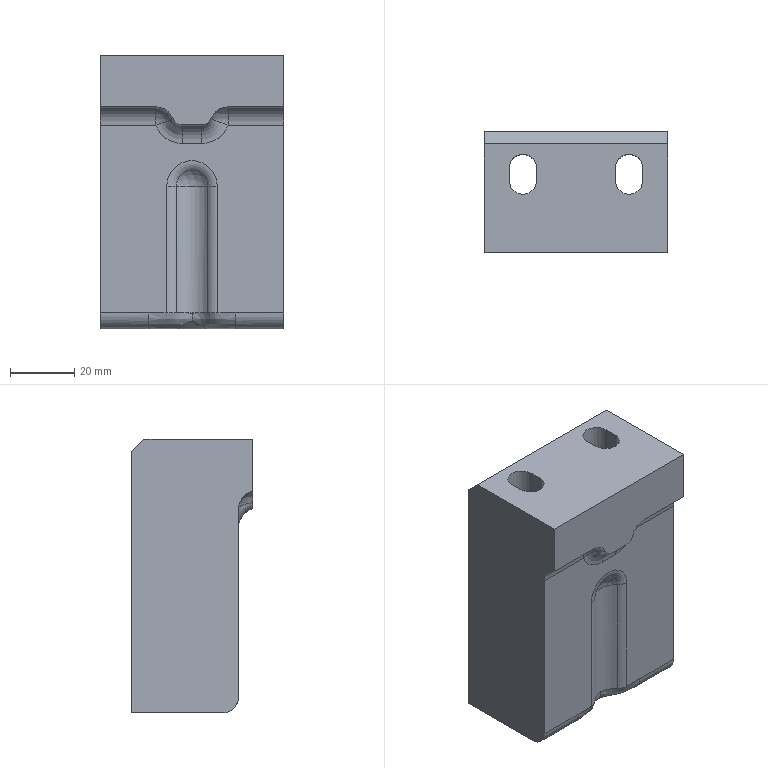Part | STEP file | 1_id54_x_t | 1 solid | 55 faces | box 57.15 x 38 x 85.5 mm | volume 141794 mm3 | plane 24 | cylinder 18 | torus 6 | sphere 3 | spline 2 | other 2 | commonest cylinder face diameters 8.5 x4 14 x4 12 x3 2 x2 8 x2 10 x2